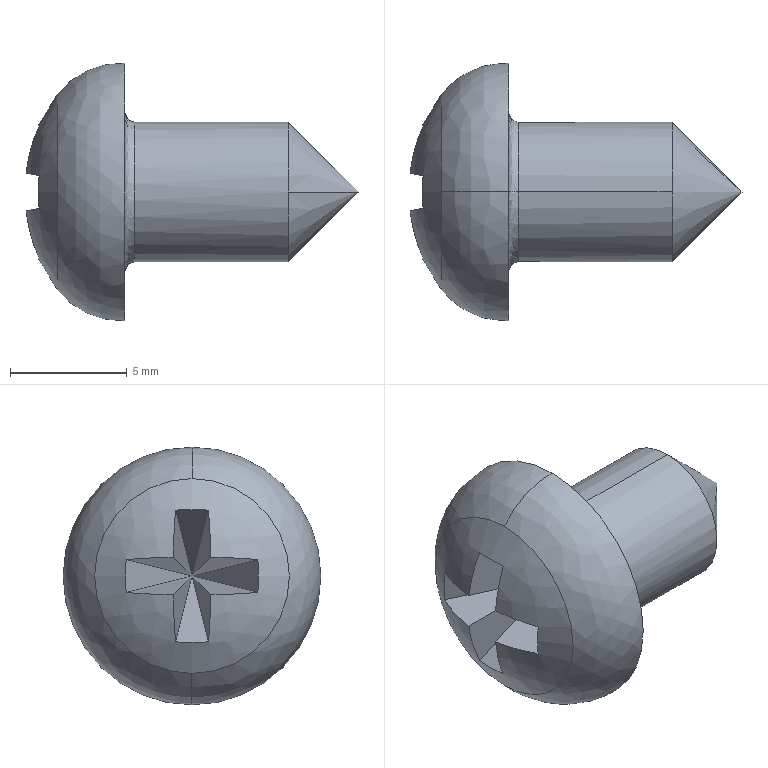Part | SolidWorks | features BaseBody 1, MoveFace 1 | 1 solid | 22 faces | box 14.243 x 11.05 x 11.056 mm | volume 485.827 mm3 | plane 13 | spline 5 | cylinder 2 | cone 2 | commonest cylinder face diameters 6 x2
STEP:
#1=CARTESIAN_POINT('',(4.74,0.,-3.));
#2=VERTEX_POINT('',#1);
#3=CARTESIAN_POINT('',(4.74,0.,3.));
#4=VERTEX_POINT('',#3);
#5=CARTESIAN_POINT('',(4.74,0.,0.));
#6=DIRECTION('',(1.,0.,0.));
#7=DIRECTION('',(0.,0.,1.));
#8=AXIS2_PLACEMENT_3D('',#5,#6,#7);
#9=CIRCLE('',#8,3.);
#10=EDGE_CURVE('',#2,#4,#9,.T.);
#11=ORIENTED_EDGE('',*,*,#10,.F.);
#12=CARTESIAN_POINT('',(4.34,0.,-3.4));
#13=VERTEX_POINT('',#12);
#14=CARTESIAN_POINT('',(4.74,0.,-3.4));
#15=DIRECTION('',(0.,-1.,0.));
#16=DIRECTION('',(0.,0.,-1.));
#17=AXIS2_PLACEMENT_3D('',#14,#15,#16);
#18=CIRCLE('',#17,0.4);
#19=EDGE_CURVE('',#2,#13,#18,.T.);
#20=ORIENTED_EDGE('',*,*,#19,.T.);
#21=CARTESIAN_POINT('',(4.34,0.,3.4));
#22=VERTEX_POINT('',#21);
#23=CARTESIAN_POINT('',(4.34,0.,3.4));
#24=CARTESIAN_POINT('',(4.34,0.2163,3.4));
#25=CARTESIAN_POINT('',(4.34,0.5349,3.37));
#26=CARTESIAN_POINT('',(4.34,0.8966,3.283));
#27=CARTESIAN_POINT('',(4.34,1.075,3.227));
#28=CARTESIAN_POINT('',(4.34,1.163,3.195));
#29=CARTESIAN_POINT('',(4.34,1.201,3.181));
#30=CARTESIAN_POINT('',(4.34,1.226,3.171));
#31=CARTESIAN_POINT('',(4.34,1.238,3.167));
#32=CARTESIAN_POINT('',(4.34,1.688,2.988));
#33=CARTESIAN_POINT('',(4.34,2.072,2.736));
#34=CARTESIAN_POINT('',(4.34,2.57,2.238));
#35=CARTESIAN_POINT('',(4.34,2.789,1.969));
#36=CARTESIAN_POINT('',(4.34,2.993,1.622));
#37=CARTESIAN_POINT('',(4.34,3.081,1.44));
#38=CARTESIAN_POINT('',(4.34,3.122,1.346));
#39=CARTESIAN_POINT('',(4.34,3.139,1.306));
#40=CARTESIAN_POINT('',(4.34,3.15,1.279));
#41=CARTESIAN_POINT('',(4.34,3.156,1.264));
#42=CARTESIAN_POINT('',(4.34,3.32,0.8492));
#43=CARTESIAN_POINT('',(4.34,3.4,0.4327));
#44=CARTESIAN_POINT('',(4.34,3.4,-0.2164));
#45=CARTESIAN_POINT('',(4.34,3.37,-0.5351));
#46=CARTESIAN_POINT('',(4.34,3.283,-0.8967));
#47=CARTESIAN_POINT('',(4.34,3.227,-1.075));
#48=CARTESIAN_POINT('',(4.34,3.195,-1.163));
#49=CARTESIAN_POINT('',(4.34,3.181,-1.201));
#50=CARTESIAN_POINT('',(4.34,3.171,-1.226));
#51=CARTESIAN_POINT('',(4.34,3.167,-1.238));
#52=CARTESIAN_POINT('',(4.34,2.988,-1.688));
#53=CARTESIAN_POINT('',(4.34,2.736,-2.072));
#54=CARTESIAN_POINT('',(4.34,2.238,-2.57));
#55=CARTESIAN_POINT('',(4.34,1.969,-2.789));
#56=CARTESIAN_POINT('',(4.34,1.622,-2.993));
#57=CARTESIAN_POINT('',(4.34,1.44,-3.081));
#58=CARTESIAN_POINT('',(4.34,1.346,-3.122));
#59=CARTESIAN_POINT('',(4.34,1.306,-3.139));
#60=CARTESIAN_POINT('',(4.34,1.279,-3.15));
#61=CARTESIAN_POINT('',(4.34,1.264,-3.156));
#62=CARTESIAN_POINT('',(4.34,0.8493,-3.32));
#63=CARTESIAN_POINT('',(4.34,0.4322,-3.4));
#64=CARTESIAN_POINT('',(4.34,0.,-3.4));
#65=B_SPLINE_CURVE_WITH_KNOTS('',3,(#23,#24,#25,#26,#27,#28,#29,#30,#31,#32,#33,#34,#35,#36,#37,#38,#39,#40,#41,#42,#43,#44,#45,#46,#47,#48,#49,#50,#51,#52,#53,#54,#55,#56,#57,#58,#59,#60,#61,#62,#63,#64),.UNSPECIFIED.,.F.,.F.,(4,1,1,1,1,2,2,2,1,1,1,1,2,2,2,1,1,1,1,2,2,2,1,1,1,1,2,2,4),(0.,0.0625,0.09375,0.1094,0.1172,0.1211,0.125,0.25,0.3125,0.3437,0.3594,0.3672,0.3711,0.375,0.5,0.5625,0.5937,0.6094,0.6172,0.6211,0.625,0.75,0.8125,0.8437,0.8594,0.8672,0.8711,0.875,1.),.UNSPECIFIED.);
#66=EDGE_CURVE('',#22,#13,#65,.T.);
#67=ORIENTED_EDGE('',*,*,#66,.F.);
#68=CARTESIAN_POINT('',(4.74,0.,3.4));
#69=DIRECTION('',(0.,1.,0.));
#70=DIRECTION('',(0.,0.,1.));
#71=AXIS2_PLACEMENT_3D('',#68,#69,#70);
#72=CIRCLE('',#71,0.4);
#73=EDGE_CURVE('',#4,#22,#72,.T.);
#74=ORIENTED_EDGE('',*,*,#73,.F.);
#75=EDGE_LOOP('',(#11,#20,#67,#74));
#76=FACE_OUTER_BOUND('',#75,.T.);
#77=CARTESIAN_POINT('',(4.74,0.,3.));
#78=CARTESIAN_POINT('',(4.74,6.,3.));
#79=CARTESIAN_POINT('',(4.74,6.,-3.));
#80=CARTESIAN_POINT('',(4.74,0.,-3.));
#81=CARTESIAN_POINT('',(4.506,0.,3.));
#82=CARTESIAN_POINT('',(4.506,6.,3.));
#83=CARTESIAN_POINT('',(4.506,6.,-3.));
#84=CARTESIAN_POINT('',(4.506,0.,-3.));
#85=CARTESIAN_POINT('',(4.34,0.,3.166));
#86=CARTESIAN_POINT('',(4.34,6.331,3.166));
#87=CARTESIAN_POINT('',(4.34,6.331,-3.166));
#88=CARTESIAN_POINT('',(4.34,0.,-3.166));
#89=CARTESIAN_POINT('',(4.34,0.,3.4));
#90=CARTESIAN_POINT('',(4.34,6.8,3.4));
#91=CARTESIAN_POINT('',(4.34,6.8,-3.4));
#92=CARTESIAN_POINT('',(4.34,0.,-3.4));
#93=(BOUNDED_SURFACE()B_SPLINE_SURFACE(3,3,((#77,#78,#79,#80),(#81,#82,#83,#84),(#85,#86,#87,#88),(#89,#90,#91,#92)),.UNSPECIFIED.,.F.,.F.,.F.)B_SPLINE_SURFACE_WITH_KNOTS((4,4),(4,4),(0.,1.),(0.,1.),.UNSPECIFIED.)GEOMETRIC_REPRESENTATION_ITEM()RATIONAL_B_SPLINE_SURFACE(((1.,0.3333,0.3333,1.),(0.8047,0.2682,0.2682,0.8047),(0.8047,0.2682,0.2682,0.8047),(1.,0.3333,0.3333,1.)))REPRESENTATION_ITEM('')SURFACE());
#94=ADVANCED_FACE('',(#76),#93,.F.);
#95=CARTESIAN_POINT('',(1.436,0.,4.179));
#96=VERTEX_POINT('',#95);
#97=CARTESIAN_POINT('',(1.436,0.,-4.179));
#98=VERTEX_POINT('',#97);
#99=CARTESIAN_POINT('',(1.436,0.,0.));
#100=DIRECTION('',(1.,0.,0.));
#101=DIRECTION('',(0.,0.,1.));
#102=AXIS2_PLACEMENT_3D('',#99,#100,#101);
#103=CIRCLE('',#102,4.179);
#104=EDGE_CURVE('',#96,#98,#103,.T.);
#105=ORIENTED_EDGE('',*,*,#104,.T.);
#106=CARTESIAN_POINT('',(4.34,0.,-5.525));
#107=VERTEX_POINT('',#106);
#108=CARTESIAN_POINT('',(4.197,0.,-2.028));
#109=DIRECTION('',(0.,-1.,0.));
#110=DIRECTION('',(0.,0.,-1.));
#111=AXIS2_PLACEMENT_3D('',#108,#109,#110);
#112=CIRCLE('',#111,3.5);
#113=EDGE_CURVE('',#98,#107,#112,.T.);
#114=ORIENTED_EDGE('',*,*,#113,.T.);
#115=CARTESIAN_POINT('',(4.34,0.,5.525));
#116=VERTEX_POINT('',#115);
#117=CARTESIAN_POINT('',(4.34,0.,0.));
#118=DIRECTION('',(-1.,0.,0.));
#119=DIRECTION('',(0.,0.,1.));
#120=AXIS2_PLACEMENT_3D('',#117,#118,#119);
#121=CIRCLE('',#120,5.525);
#122=EDGE_CURVE('',#107,#116,#121,.T.);
#123=ORIENTED_EDGE('',*,*,#122,.T.);
#124=CARTESIAN_POINT('',(4.197,0.,2.028));
#125=DIRECTION('',(0.,1.,0.));
#126=DIRECTION('',(0.,0.,1.));
#127=AXIS2_PLACEMENT_3D('',#124,#125,#126);
#128=CIRCLE('',#127,3.5);
#129=EDGE_CURVE('',#96,#116,#128,.T.);
#130=ORIENTED_EDGE('',*,*,#129,.F.);
#131=EDGE_LOOP('',(#105,#114,#123,#130));
#132=FACE_OUTER_BOUND('',#131,.T.);
#133=CARTESIAN_POINT('',(1.436,0.,-4.179));
#134=CARTESIAN_POINT('',(1.436,-8.358,-4.179));
#135=CARTESIAN_POINT('',(1.436,-8.358,4.179));
#136=CARTESIAN_POINT('',(1.436,0.,4.179));
#137=CARTESIAN_POINT('',(2.144,0.,-5.088));
#138=CARTESIAN_POINT('',(2.144,-10.175,-5.088));
#139=CARTESIAN_POINT('',(2.144,-10.175,5.088));
#140=CARTESIAN_POINT('',(2.144,0.,5.088));
#141=CARTESIAN_POINT('',(3.189,0.,-5.572));
#142=CARTESIAN_POINT('',(3.189,-11.144,-5.572));
#143=CARTESIAN_POINT('',(3.189,-11.144,5.572));
#144=CARTESIAN_POINT('',(3.189,0.,5.572));
#145=CARTESIAN_POINT('',(4.34,0.,-5.525));
#146=CARTESIAN_POINT('',(4.34,-11.05,-5.525));
#147=CARTESIAN_POINT('',(4.34,-11.05,5.525));
#148=CARTESIAN_POINT('',(4.34,0.,5.525));
#149=(BOUNDED_SURFACE()B_SPLINE_SURFACE(3,3,((#133,#134,#135,#136),(#137,#138,#139,#140),(#141,#142,#143,#144),(#145,#146,#147,#148)),.UNSPECIFIED.,.F.,.F.,.F.)B_SPLINE_SURFACE_WITH_KNOTS((4,4),(4,4),(0.,1.),(0.,1.),.UNSPECIFIED.)GEOMETRIC_REPRESENTATION_ITEM()RATIONAL_B_SPLINE_SURFACE(((1.,0.3333,0.3333,1.),(0.9262,0.3087,0.3087,0.9262),(0.9262,0.3087,0.3087,0.9262),(1.,0.3333,0.3333,1.)))REPRESENTATION_ITEM('')SURFACE());
#150=ADVANCED_FACE('',(#132),#149,.T.);
#151=CARTESIAN_POINT('',(11.34,3.,0.));
#152=VERTEX_POINT('',#151);
#153=CARTESIAN_POINT('',(11.34,0.,-3.));
#154=VERTEX_POINT('',#153);
#155=CARTESIAN_POINT('',(11.34,0.,0.));
#156=DIRECTION('',(-1.,0.,0.));
#157=DIRECTION('',(0.,0.,1.));
#158=AXIS2_PLACEMENT_3D('',#155,#156,#157);
#159=CIRCLE('',#158,3.);
#160=EDGE_CURVE('',#152,#154,#159,.T.);
#161=ORIENTED_EDGE('',*,*,#160,.T.);
#162=CARTESIAN_POINT('',(-13.629,0.,-3.));
#163=DIRECTION('',(-1.,0.,0.));
#164=VECTOR('',#163,1000.);
#165=LINE('',#162,#164);
#166=EDGE_CURVE('',#154,#2,#165,.T.);
#167=ORIENTED_EDGE('',*,*,#166,.T.);
#168=ORIENTED_EDGE('',*,*,#10,.T.);
#169=CARTESIAN_POINT('',(11.34,0.,3.));
#170=VERTEX_POINT('',#169);
#171=CARTESIAN_POINT('',(-13.629,0.,3.));
#172=DIRECTION('',(-1.,0.,0.));
#173=VECTOR('',#172,1000.);
#174=LINE('',#171,#173);
#175=EDGE_CURVE('',#170,#4,#174,.T.);
#176=ORIENTED_EDGE('',*,*,#175,.F.);
#177=CARTESIAN_POINT('',(11.34,0.,0.));
#178=DIRECTION('',(-1.,0.,0.));
#179=DIRECTION('',(0.,0.,1.));
#180=AXIS2_PLACEMENT_3D('',#177,#178,#179);
#181=CIRCLE('',#180,3.);
#182=EDGE_CURVE('',#170,#152,#181,.T.);
#183=ORIENTED_EDGE('',*,*,#182,.T.);
#184=EDGE_LOOP('',(#161,#167,#168,#176,#183));
#185=FACE_OUTER_BOUND('',#184,.T.);
#186=CARTESIAN_POINT('',(-13.629,0.,0.));
#187=DIRECTION('',(-1.,0.,0.));
#188=DIRECTION('',(0.,0.,1.));
#189=AXIS2_PLACEMENT_3D('',#186,#187,#188);
#190=CYLINDRICAL_SURFACE('',#189,3.);
#191=ADVANCED_FACE('',(#185),#190,.T.);
#192=CARTESIAN_POINT('',(14.34,0.,0.));
#193=VERTEX_POINT('',#192);
#194=CARTESIAN_POINT('',(11.34,-3.,0.));
#195=VERTEX_POINT('',#194);
#196=CARTESIAN_POINT('',(11.34,-3.,0.));
#197=DIRECTION('',(-0.7071,-0.7071,0.));
#198=VECTOR('',#197,1000.);
#199=LINE('',#196,#198);
#200=EDGE_CURVE('',#193,#195,#199,.T.);
#201=ORIENTED_EDGE('',*,*,#200,.F.);
#202=CARTESIAN_POINT('',(11.34,3.,0.));
#203=DIRECTION('',(-0.7071,0.7071,0.));
#204=VECTOR('',#203,1000.);
#205=LINE('',#202,#204);
#206=EDGE_CURVE('',#193,#152,#205,.T.);
#207=ORIENTED_EDGE('',*,*,#206,.T.);
#208=ORIENTED_EDGE('',*,*,#182,.F.);
#209=CARTESIAN_POINT('',(11.34,0.,0.));
#210=DIRECTION('',(-1.,0.,0.));
#211=DIRECTION('',(0.,0.,1.));
#212=AXIS2_PLACEMENT_3D('',#209,#210,#211);
#213=CIRCLE('',#212,3.);
#214=EDGE_CURVE('',#195,#170,#213,.T.);
#215=ORIENTED_EDGE('',*,*,#214,.F.);
#216=EDGE_LOOP('',(#201,#207,#208,#215));
#217=FACE_OUTER_BOUND('',#216,.T.);
#218=CARTESIAN_POINT('',(11.34,0.,0.));
#219=DIRECTION('',(-1.,0.,0.));
#220=DIRECTION('',(0.,-1.,0.));
#221=AXIS2_PLACEMENT_3D('',#218,#219,#220);
#222=CONICAL_SURFACE('',#221,3.,0.7854);
#223=ADVANCED_FACE('',(#217),#222,.T.);
#224=ORIENTED_EDGE('',*,*,#166,.F.);
#225=CARTESIAN_POINT('',(11.34,0.,0.));
#226=DIRECTION('',(-1.,0.,0.));
#227=DIRECTION('',(0.,0.,1.));
#228=AXIS2_PLACEMENT_3D('',#225,#226,#227);
#229=CIRCLE('',#228,3.);
#230=EDGE_CURVE('',#154,#195,#229,.T.);
#231=ORIENTED_EDGE('',*,*,#230,.T.);
#232=ORIENTED_EDGE('',*,*,#214,.T.);
#233=ORIENTED_EDGE('',*,*,#175,.T.);
#234=CARTESIAN_POINT('',(4.74,0.,0.));
#235=DIRECTION('',(1.,0.,0.));
#236=DIRECTION('',(0.,0.,1.));
#237=AXIS2_PLACEMENT_3D('',#234,#235,#236);
#238=CIRCLE('',#237,3.);
#239=EDGE_CURVE('',#4,#2,#238,.T.);
#240=ORIENTED_EDGE('',*,*,#239,.T.);
#241=EDGE_LOOP('',(#224,#231,#232,#233,#240));
#242=FACE_OUTER_BOUND('',#241,.T.);
#243=CARTESIAN_POINT('',(-13.629,0.,0.));
#244=DIRECTION('',(-1.,0.,0.));
#245=DIRECTION('',(0.,0.,1.));
#246=AXIS2_PLACEMENT_3D('',#243,#244,#245);
#247=CYLINDRICAL_SURFACE('',#246,3.);
#248=ADVANCED_FACE('',(#242),#247,.T.);
#249=ORIENTED_EDGE('',*,*,#19,.F.);
#250=ORIENTED_EDGE('',*,*,#239,.F.);
#251=ORIENTED_EDGE('',*,*,#73,.T.);
#252=CARTESIAN_POINT('',(4.34,0.,-3.4));
#253=CARTESIAN_POINT('',(4.34,-0.2163,-3.4));
#254=CARTESIAN_POINT('',(4.34,-0.5349,-3.37));
#255=CARTESIAN_POINT('',(4.34,-0.8966,-3.283));
#256=CARTESIAN_POINT('',(4.34,-1.075,-3.227));
#257=CARTESIAN_POINT('',(4.34,-1.163,-3.195));
#258=CARTESIAN_POINT('',(4.34,-1.201,-3.181));
#259=CARTESIAN_POINT('',(4.34,-1.226,-3.171));
#260=CARTESIAN_POINT('',(4.34,-1.238,-3.167));
#261=CARTESIAN_POINT('',(4.34,-1.688,-2.988));
#262=CARTESIAN_POINT('',(4.34,-2.072,-2.736));
#263=CARTESIAN_POINT('',(4.34,-2.57,-2.238));
#264=CARTESIAN_POINT('',(4.34,-2.789,-1.969));
#265=CARTESIAN_POINT('',(4.34,-2.993,-1.622));
#266=CARTESIAN_POINT('',(4.34,-3.081,-1.44));
#267=CARTESIAN_POINT('',(4.34,-3.122,-1.346));
#268=CARTESIAN_POINT('',(4.34,-3.139,-1.306));
#269=CARTESIAN_POINT('',(4.34,-3.15,-1.279));
#270=CARTESIAN_POINT('',(4.34,-3.156,-1.264));
#271=CARTESIAN_POINT('',(4.34,-3.32,-0.8492));
#272=CARTESIAN_POINT('',(4.34,-3.4,-0.4327));
#273=CARTESIAN_POINT('',(4.34,-3.4,0.2164));
#274=CARTESIAN_POINT('',(4.34,-3.37,0.5351));
#275=CARTESIAN_POINT('',(4.34,-3.283,0.8967));
#276=CARTESIAN_POINT('',(4.34,-3.227,1.075));
#277=CARTESIAN_POINT('',(4.34,-3.195,1.163));
#278=CARTESIAN_POINT('',(4.34,-3.181,1.201));
#279=CARTESIAN_POINT('',(4.34,-3.171,1.226));
#280=CARTESIAN_POINT('',(4.34,-3.167,1.238));
#281=CARTESIAN_POINT('',(4.34,-2.988,1.688));
#282=CARTESIAN_POINT('',(4.34,-2.736,2.072));
#283=CARTESIAN_POINT('',(4.34,-2.238,2.57));
#284=CARTESIAN_POINT('',(4.34,-1.969,2.789));
#285=CARTESIAN_POINT('',(4.34,-1.622,2.993));
#286=CARTESIAN_POINT('',(4.34,-1.44,3.081));
#287=CARTESIAN_POINT('',(4.34,-1.346,3.122));
#288=CARTESIAN_POINT('',(4.34,-1.306,3.139));
#289=CARTESIAN_POINT('',(4.34,-1.279,3.15));
#290=CARTESIAN_POINT('',(4.34,-1.264,3.156));
#291=CARTESIAN_POINT('',(4.34,-0.8493,3.32));
#292=CARTESIAN_POINT('',(4.34,-0.4322,3.4));
#293=CARTESIAN_POINT('',(4.34,0.,3.4));
#294=B_SPLINE_CURVE_WITH_KNOTS('',3,(#252,#253,#254,#255,#256,#257,#258,#259,#260,#261,#262,#263,#264,#265,#266,#267,#268,#269,#270,#271,#272,#273,#274,#275,#276,#277,#278,#279,#280,#281,#282,#283,#284,#285,#286,#287,#288,#289,#290,#291,#292,#293),.UNSPECIFIED.,.F.,.F.,(4,1,1,1,1,2,2,2,1,1,1,1,2,2,2,1,1,1,1,2,2,2,1,1,1,1,2,2,4),(0.,0.0625,0.09375,0.1094,0.1172,0.1211,0.125,0.25,0.3125,0.3437,0.3594,0.3672,0.3711,0.375,0.5,0.5625,0.5937,0.6094,0.6172,0.6211,0.625,0.75,0.8125,0.8437,0.8594,0.8672,0.8711,0.875,1.),.UNSPECIFIED.);
#295=EDGE_CURVE('',#13,#22,#294,.T.);
#296=ORIENTED_EDGE('',*,*,#295,.F.);
#297=EDGE_LOOP('',(#249,#250,#251,#296));
#298=FACE_OUTER_BOUND('',#297,.T.);
#299=CARTESIAN_POINT('',(4.74,0.,-3.));
#300=CARTESIAN_POINT('',(4.74,-6.,-3.));
#301=CARTESIAN_POINT('',(4.74,-6.,3.));
#302=CARTESIAN_POINT('',(4.74,0.,3.));
#303=CARTESIAN_POINT('',(4.506,0.,-3.));
#304=CARTESIAN_POINT('',(4.506,-6.,-3.));
#305=CARTESIAN_POINT('',(4.506,-6.,3.));
#306=CARTESIAN_POINT('',(4.506,0.,3.));
#307=CARTESIAN_POINT('',(4.34,0.,-3.166));
#308=CARTESIAN_POINT('',(4.34,-6.331,-3.166));
#309=CARTESIAN_POINT('',(4.34,-6.331,3.166));
#310=CARTESIAN_POINT('',(4.34,0.,3.166));
#311=CARTESIAN_POINT('',(4.34,0.,-3.4));
#312=CARTESIAN_POINT('',(4.34,-6.8,-3.4));
#313=CARTESIAN_POINT('',(4.34,-6.8,3.4));
#314=CARTESIAN_POINT('',(4.34,0.,3.4));
#315=(BOUNDED_SURFACE()B_SPLINE_SURFACE(3,3,((#299,#300,#301,#302),(#303,#304,#305,#306),(#307,#308,#309,#310),(#311,#312,#313,#314)),.UNSPECIFIED.,.F.,.F.,.F.)B_SPLINE_SURFACE_WITH_KNOTS((4,4),(4,4),(0.,1.),(0.,1.),.UNSPECIFIED.)GEOMETRIC_REPRESENTATION_ITEM()RATIONAL_B_SPLINE_SURFACE(((1.,0.3333,0.3333,1.),(0.8047,0.2682,0.2682,0.8047),(0.8047,0.2682,0.2682,0.8047),(1.,0.3333,0.3333,1.)))REPRESENTATION_ITEM('')SURFACE());
#316=ADVANCED_FACE('',(#298),#315,.F.);
#317=ORIENTED_EDGE('',*,*,#206,.F.);
#318=ORIENTED_EDGE('',*,*,#200,.T.);
#319=ORIENTED_EDGE('',*,*,#230,.F.);
#320=ORIENTED_EDGE('',*,*,#160,.F.);
#321=EDGE_LOOP('',(#317,#318,#319,#320));
#322=FACE_OUTER_BOUND('',#321,.T.);
#323=CARTESIAN_POINT('',(11.34,0.,0.));
#324=DIRECTION('',(-1.,0.,0.));
#325=DIRECTION('',(0.,-1.,0.));
#326=AXIS2_PLACEMENT_3D('',#323,#324,#325);
#327=CONICAL_SURFACE('',#326,3.,0.7854);
#328=ADVANCED_FACE('',(#322),#327,.T.);
#329=CARTESIAN_POINT('',(4.34,0.,0.));
#330=DIRECTION('',(-1.,0.,0.));
#331=DIRECTION('',(0.,0.,1.));
#332=AXIS2_PLACEMENT_3D('',#329,#330,#331);
#333=CIRCLE('',#332,5.525);
#334=EDGE_CURVE('',#116,#107,#333,.T.);
#335=ORIENTED_EDGE('',*,*,#334,.F.);
#336=ORIENTED_EDGE('',*,*,#122,.F.);
#337=EDGE_LOOP('',(#335,#336));
#338=FACE_OUTER_BOUND('',#337,.T.);
#339=ORIENTED_EDGE('',*,*,#295,.T.);
#340=ORIENTED_EDGE('',*,*,#66,.T.);
#341=EDGE_LOOP('',(#339,#340));
#342=FACE_BOUND('',#341,.T.);
#343=CARTESIAN_POINT('',(4.34,0.,-3.));
#344=DIRECTION('',(-1.,0.,0.));
#345=DIRECTION('',(0.,0.,1.));
#346=AXIS2_PLACEMENT_3D('',#343,#344,#345);
#347=PLANE('',#346);
#348=ADVANCED_FACE('',(#338,#342),#347,.F.);
#349=ORIENTED_EDGE('',*,*,#113,.F.);
#350=CARTESIAN_POINT('',(1.436,0.,0.));
#351=DIRECTION('',(1.,0.,0.));
#352=DIRECTION('',(0.,0.,1.));
#353=AXIS2_PLACEMENT_3D('',#350,#351,#352);
#354=CIRCLE('',#353,4.179);
#355=EDGE_CURVE('',#98,#96,#354,.T.);
#356=ORIENTED_EDGE('',*,*,#355,.T.);
#357=ORIENTED_EDGE('',*,*,#129,.T.);
#358=ORIENTED_EDGE('',*,*,#334,.T.);
#359=EDGE_LOOP('',(#349,#356,#357,#358));
#360=FACE_OUTER_BOUND('',#359,.T.);
#361=CARTESIAN_POINT('',(1.436,0.,4.179));
#362=CARTESIAN_POINT('',(1.436,8.358,4.179));
#363=CARTESIAN_POINT('',(1.436,8.358,-4.179));
#364=CARTESIAN_POINT('',(1.436,0.,-4.179));
#365=CARTESIAN_POINT('',(2.144,0.,5.088));
#366=CARTESIAN_POINT('',(2.144,10.175,5.088));
#367=CARTESIAN_POINT('',(2.144,10.175,-5.088));
#368=CARTESIAN_POINT('',(2.144,0.,-5.088));
#369=CARTESIAN_POINT('',(3.189,0.,5.572));
#370=CARTESIAN_POINT('',(3.189,11.144,5.572));
#371=CARTESIAN_POINT('',(3.189,11.144,-5.572));
#372=CARTESIAN_POINT('',(3.189,0.,-5.572));
#373=CARTESIAN_POINT('',(4.34,0.,5.525));
#374=CARTESIAN_POINT('',(4.34,11.05,5.525));
#375=CARTESIAN_POINT('',(4.34,11.05,-5.525));
#376=CARTESIAN_POINT('',(4.34,0.,-5.525));
#377=(BOUNDED_SURFACE()B_SPLINE_SURFACE(3,3,((#361,#362,#363,#364),(#365,#366,#367,#368),(#369,#370,#371,#372),(#373,#374,#375,#376)),.UNSPECIFIED.,.F.,.F.,.F.)B_SPLINE_SURFACE_WITH_KNOTS((4,4),(4,4),(0.,1.),(0.,1.),.UNSPECIFIED.)GEOMETRIC_REPRESENTATION_ITEM()RATIONAL_B_SPLINE_SURFACE(((1.,0.3333,0.3333,1.),(0.9262,0.3087,0.3087,0.9262),(0.9262,0.3087,0.3087,0.9262),(1.,0.3333,0.3333,1.)))REPRESENTATION_ITEM('')SURFACE());
#378=ADVANCED_FACE('',(#360),#377,.T.);
#379=ORIENTED_EDGE('',*,*,#104,.F.);
#380=ORIENTED_EDGE('',*,*,#355,.F.);
#381=EDGE_LOOP('',(#379,#380));
#382=FACE_OUTER_BOUND('',#381,.T.);
#383=CARTESIAN_POINT('',(0.09661,0.8076,0.8076));
#384=VERTEX_POINT('',#383);
#385=CARTESIAN_POINT('',(0.6565,0.707,2.828));
#386=VERTEX_POINT('',#385);
#387=CARTESIAN_POINT('',(0.09661,0.8076,0.8076));
#388=CARTESIAN_POINT('',(0.1795,0.7927,1.511));
#389=CARTESIAN_POINT('',(0.3662,0.7592,2.184));
#390=CARTESIAN_POINT('',(0.6565,0.707,2.828));
#391=B_SPLINE_CURVE_WITH_KNOTS('',3,(#387,#388,#389,#390),.UNSPECIFIED.,.F.,.F.,(4,4),(0.,0.002099),.UNSPECIFIED.);
#392=EDGE_CURVE('',#384,#386,#391,.T.);
#393=ORIENTED_EDGE('',*,*,#392,.T.);
#394=CARTESIAN_POINT('',(0.6565,-0.707,2.828));
#395=VERTEX_POINT('',#394);
#396=CARTESIAN_POINT('',(0.6565,0.707,2.828));
#397=CARTESIAN_POINT('',(0.6159,0.237,2.857));
#398=CARTESIAN_POINT('',(0.6159,-0.237,2.857));
#399=CARTESIAN_POINT('',(0.6565,-0.707,2.828));
#400=B_SPLINE_CURVE_WITH_KNOTS('',3,(#396,#397,#398,#399),.UNSPECIFIED.,.F.,.F.,(4,4),(-0.000708,0.000708),.UNSPECIFIED.);
#401=EDGE_CURVE('',#386,#395,#400,.T.);
#402=ORIENTED_EDGE('',*,*,#401,.T.);
#403=CARTESIAN_POINT('',(0.09661,-0.8076,0.8076));
#404=VERTEX_POINT('',#403);
#405=CARTESIAN_POINT('',(0.6565,-0.707,2.828));
#406=CARTESIAN_POINT('',(0.3662,-0.7592,2.184));
#407=CARTESIAN_POINT('',(0.1795,-0.7927,1.511));
#408=CARTESIAN_POINT('',(0.09661,-0.8076,0.8076));
#409=B_SPLINE_CURVE_WITH_KNOTS('',3,(#405,#406,#407,#408),.UNSPECIFIED.,.F.,.F.,(4,4),(0.,0.002099),.UNSPECIFIED.);
#410=EDGE_CURVE('',#395,#404,#409,.T.);
#411=ORIENTED_EDGE('',*,*,#410,.T.);
#412=CARTESIAN_POINT('',(0.6565,-2.828,0.707));
#413=VERTEX_POINT('',#412);
#414=CARTESIAN_POINT('',(0.09661,-0.8076,0.8076));
#415=CARTESIAN_POINT('',(0.1795,-1.511,0.7927));
#416=CARTESIAN_POINT('',(0.3662,-2.184,0.7592));
#417=CARTESIAN_POINT('',(0.6565,-2.828,0.707));
#418=B_SPLINE_CURVE_WITH_KNOTS('',3,(#414,#415,#416,#417),.UNSPECIFIED.,.F.,.F.,(4,4),(0.,0.002099),.UNSPECIFIED.);
#419=EDGE_CURVE('',#404,#413,#418,.T.);
#420=ORIENTED_EDGE('',*,*,#419,.T.);
#421=CARTESIAN_POINT('',(0.6565,-2.828,-0.707));
#422=VERTEX_POINT('',#421);
#423=CARTESIAN_POINT('',(0.6565,-2.828,0.707));
#424=CARTESIAN_POINT('',(0.6157,-2.857,0.2357));
#425=CARTESIAN_POINT('',(0.6157,-2.857,-0.2357));
#426=CARTESIAN_POINT('',(0.6565,-2.828,-0.707));
#427=B_SPLINE_CURVE_WITH_KNOTS('',3,(#423,#424,#425,#426),.UNSPECIFIED.,.F.,.F.,(4,4),(0.,0.001414),.UNSPECIFIED.);
#428=EDGE_CURVE('',#413,#422,#427,.T.);
#429=ORIENTED_EDGE('',*,*,#428,.T.);
#430=CARTESIAN_POINT('',(0.09661,-0.8076,-0.8076));
#431=VERTEX_POINT('',#430);
#432=CARTESIAN_POINT('',(0.6565,-2.828,-0.707));
#433=CARTESIAN_POINT('',(0.3662,-2.184,-0.7592));
#434=CARTESIAN_POINT('',(0.1795,-1.511,-0.7927));
#435=CARTESIAN_POINT('',(0.09661,-0.8076,-0.8076));
#436=B_SPLINE_CURVE_WITH_KNOTS('',3,(#432,#433,#434,#435),.UNSPECIFIED.,.F.,.F.,(4,4),(0.,0.002099),.UNSPECIFIED.);
#437=EDGE_CURVE('',#422,#431,#436,.T.);
#438=ORIENTED_EDGE('',*,*,#437,.T.);
#439=CARTESIAN_POINT('',(0.6565,-0.707,-2.828));
#440=VERTEX_POINT('',#439);
#441=CARTESIAN_POINT('',(0.09661,-0.8076,-0.8076));
#442=CARTESIAN_POINT('',(0.1795,-0.7927,-1.511));
#443=CARTESIAN_POINT('',(0.3662,-0.7592,-2.184));
#444=CARTESIAN_POINT('',(0.6565,-0.707,-2.828));
#445=B_SPLINE_CURVE_WITH_KNOTS('',3,(#441,#442,#443,#444),.UNSPECIFIED.,.F.,.F.,(4,4),(0.,0.002099),.UNSPECIFIED.);
#446=EDGE_CURVE('',#431,#440,#445,.T.);
#447=ORIENTED_EDGE('',*,*,#446,.T.);
#448=CARTESIAN_POINT('',(0.6565,0.707,-2.828));
#449=VERTEX_POINT('',#448);
#450=CARTESIAN_POINT('',(0.6565,-0.707,-2.828));
#451=CARTESIAN_POINT('',(0.6159,-0.237,-2.857));
#452=CARTESIAN_POINT('',(0.6159,0.237,-2.857));
#453=CARTESIAN_POINT('',(0.6565,0.707,-2.828));
#454=B_SPLINE_CURVE_WITH_KNOTS('',3,(#450,#451,#452,#453),.UNSPECIFIED.,.F.,.F.,(4,4),(-0.000708,0.000708),.UNSPECIFIED.);
#455=EDGE_CURVE('',#440,#449,#454,.T.);
#456=ORIENTED_EDGE('',*,*,#455,.T.);
#457=CARTESIAN_POINT('',(0.09661,0.8076,-0.8076));
#458=VERTEX_POINT('',#457);
#459=CARTESIAN_POINT('',(0.6565,0.707,-2.828));
#460=CARTESIAN_POINT('',(0.3662,0.7592,-2.184));
#461=CARTESIAN_POINT('',(0.1795,0.7927,-1.511));
#462=CARTESIAN_POINT('',(0.09661,0.8076,-0.8076));
#463=B_SPLINE_CURVE_WITH_KNOTS('',3,(#459,#460,#461,#462),.UNSPECIFIED.,.F.,.F.,(4,4),(0.,0.002099),.UNSPECIFIED.);
#464=EDGE_CURVE('',#449,#458,#463,.T.);
#465=ORIENTED_EDGE('',*,*,#464,.T.);
#466=CARTESIAN_POINT('',(0.6565,2.828,-0.707));
#467=VERTEX_POINT('',#466);
#468=CARTESIAN_POINT('',(0.09661,0.8076,-0.8076));
#469=CARTESIAN_POINT('',(0.1795,1.511,-0.7927));
#470=CARTESIAN_POINT('',(0.3662,2.184,-0.7592));
#471=CARTESIAN_POINT('',(0.6565,2.828,-0.707));
#472=B_SPLINE_CURVE_WITH_KNOTS('',3,(#468,#469,#470,#471),.UNSPECIFIED.,.F.,.F.,(4,4),(0.,0.002099),.UNSPECIFIED.);
#473=EDGE_CURVE('',#458,#467,#472,.T.);
#474=ORIENTED_EDGE('',*,*,#473,.T.);
#475=CARTESIAN_POINT('',(0.6565,2.828,0.707));
#476=VERTEX_POINT('',#475);
#477=CARTESIAN_POINT('',(0.6565,2.828,-0.707));
#478=CARTESIAN_POINT('',(0.6157,2.857,-0.2357));
#479=CARTESIAN_POINT('',(0.6157,2.857,0.2357));
#480=CARTESIAN_POINT('',(0.6565,2.828,0.707));
#481=B_SPLINE_CURVE_WITH_KNOTS('',3,(#477,#478,#479,#480),.UNSPECIFIED.,.F.,.F.,(4,4),(0.,0.001414),.UNSPECIFIED.);
#482=EDGE_CURVE('',#467,#476,#481,.T.);
#483=ORIENTED_EDGE('',*,*,#482,.T.);
#484=CARTESIAN_POINT('',(0.6565,2.828,0.707));
#485=CARTESIAN_POINT('',(0.3662,2.184,0.7592));
#486=CARTESIAN_POINT('',(0.1795,1.511,0.7927));
#487=CARTESIAN_POINT('',(0.09661,0.8076,0.8076));
#488=B_SPLINE_CURVE_WITH_KNOTS('',3,(#484,#485,#486,#487),.UNSPECIFIED.,.F.,.F.,(4,4),(0.,0.002099),.UNSPECIFIED.);
#489=EDGE_CURVE('',#476,#384,#488,.T.);
#490=ORIENTED_EDGE('',*,*,#489,.T.);
#491=EDGE_LOOP('',(#393,#402,#411,#420,#429,#438,#447,#456,#465,#474,#483,#490));
#492=FACE_BOUND('',#491,.T.);
#493=CARTESIAN_POINT('',(2.642,-3.304,-4.246));
#494=CARTESIAN_POINT('',(1.037,-1.284,-4.246));
#495=CARTESIAN_POINT('',(1.039,1.296,-4.246));
#496=CARTESIAN_POINT('',(2.649,3.313,-4.246));
#497=CARTESIAN_POINT('',(1.028,-4.587,-1.668));
#498=CARTESIAN_POINT('',(-1.2,-1.782,-1.668));
#499=CARTESIAN_POINT('',(-1.197,1.799,-1.668));
#500=CARTESIAN_POINT('',(1.037,4.599,-1.668));
#501=CARTESIAN_POINT('',(1.022,-4.591,1.633));
#502=CARTESIAN_POINT('',(-1.209,-1.784,1.633));
#503=CARTESIAN_POINT('',(-1.205,1.801,1.633));
#504=CARTESIAN_POINT('',(1.031,4.604,1.633));
#505=CARTESIAN_POINT('',(2.626,-3.316,4.221));
#506=CARTESIAN_POINT('',(1.015,-1.289,4.221));
#507=CARTESIAN_POINT('',(1.018,1.301,4.221));
#508=CARTESIAN_POINT('',(2.633,3.325,4.221));
#509=(BOUNDED_SURFACE()B_SPLINE_SURFACE(3,3,((#493,#494,#495,#496),(#497,#498,#499,#500),(#501,#502,#503,#504),(#505,#506,#507,#508)),.UNSPECIFIED.,.F.,.F.,.T.)B_SPLINE_SURFACE_WITH_KNOTS((4,4),(4,4),(0.,1.),(0.,1.),.UNSPECIFIED.)GEOMETRIC_REPRESENTATION_ITEM()RATIONAL_B_SPLINE_SURFACE(((1.,0.8549,0.8549,1.),(0.855,0.7309,0.7309,0.855),(0.855,0.7309,0.7309,0.855),(1.,0.8549,0.8549,1.)))REPRESENTATION_ITEM('')SURFACE());
#510=ADVANCED_FACE('',(#382,#492),#509,.T.);
#511=CARTESIAN_POINT('',(4.59,0.,0.));
#512=VERTEX_POINT('',#511);
#513=CARTESIAN_POINT('',(0.6565,0.707,2.828));
#514=DIRECTION('',(0.8034,-0.1444,-0.5776));
#515=VECTOR('',#514,1000.);
#516=LINE('',#513,#515);
#517=EDGE_CURVE('',#386,#512,#516,.T.);
#518=ORIENTED_EDGE('',*,*,#517,.F.);
#519=ORIENTED_EDGE('',*,*,#392,.F.);
#520=CARTESIAN_POINT('',(4.59,0.,0.));
#521=DIRECTION('',(-0.9692,0.1742,0.1742));
#522=VECTOR('',#521,1000.);
#523=LINE('',#520,#522);
#524=EDGE_CURVE('',#512,#384,#523,.T.);
#525=ORIENTED_EDGE('',*,*,#524,.F.);
#526=EDGE_LOOP('',(#518,#519,#525));
#527=FACE_OUTER_BOUND('',#526,.T.);
#528=CARTESIAN_POINT('',(0.,0.825,0.825));
#529=DIRECTION('',(0.1769,0.9842,0.));
#530=DIRECTION('',(-0.9842,0.1769,0.));
#531=AXIS2_PLACEMENT_3D('',#528,#529,#530);
#532=PLANE('',#531);
#533=ADVANCED_FACE('',(#527),#532,.F.);
#534=ORIENTED_EDGE('',*,*,#524,.T.);
#535=ORIENTED_EDGE('',*,*,#489,.F.);
#536=CARTESIAN_POINT('',(4.59,0.,0.));
#537=DIRECTION('',(-0.8034,0.5776,0.1444));
#538=VECTOR('',#537,1000.);
#539=LINE('',#536,#538);
#540=EDGE_CURVE('',#512,#476,#539,.T.);
#541=ORIENTED_EDGE('',*,*,#540,.F.);
#542=EDGE_LOOP('',(#534,#535,#541));
#543=FACE_OUTER_BOUND('',#542,.T.);
#544=CARTESIAN_POINT('',(0.,3.3,0.825));
#545=DIRECTION('',(0.1769,0.,0.9842));
#546=DIRECTION('',(0.9842,0.,-0.1769));
#547=AXIS2_PLACEMENT_3D('',#544,#545,#546);
#548=PLANE('',#547);
#549=ADVANCED_FACE('',(#543),#548,.F.);
#550=CARTESIAN_POINT('',(0.6565,2.828,-0.707));
#551=DIRECTION('',(0.8034,-0.5776,0.1444));
#552=VECTOR('',#551,1000.);
#553=LINE('',#550,#552);
#554=EDGE_CURVE('',#467,#512,#553,.T.);
#555=ORIENTED_EDGE('',*,*,#554,.F.);
#556=ORIENTED_EDGE('',*,*,#473,.F.);
#557=CARTESIAN_POINT('',(4.59,0.,0.));
#558=DIRECTION('',(-0.9692,0.1742,-0.1742));
#559=VECTOR('',#558,1000.);
#560=LINE('',#557,#559);
#561=EDGE_CURVE('',#512,#458,#560,.T.);
#562=ORIENTED_EDGE('',*,*,#561,.F.);
#563=EDGE_LOOP('',(#555,#556,#562));
#564=FACE_OUTER_BOUND('',#563,.T.);
#565=CARTESIAN_POINT('',(0.,0.825,-0.825));
#566=DIRECTION('',(0.1769,0.,-0.9842));
#567=DIRECTION('',(-0.9842,0.,-0.1769));
#568=AXIS2_PLACEMENT_3D('',#565,#566,#567);
#569=PLANE('',#568);
#570=ADVANCED_FACE('',(#564),#569,.F.);
#571=ORIENTED_EDGE('',*,*,#561,.T.);
#572=ORIENTED_EDGE('',*,*,#464,.F.);
#573=CARTESIAN_POINT('',(4.59,0.,0.));
#574=DIRECTION('',(-0.8034,0.1444,-0.5776));
#575=VECTOR('',#574,1000.);
#576=LINE('',#573,#575);
#577=EDGE_CURVE('',#512,#449,#576,.T.);
#578=ORIENTED_EDGE('',*,*,#577,.F.);
#579=EDGE_LOOP('',(#571,#572,#578));
#580=FACE_OUTER_BOUND('',#579,.T.);
#581=CARTESIAN_POINT('',(0.,0.825,-3.3));
#582=DIRECTION('',(0.1769,0.9842,0.));
#583=DIRECTION('',(-0.9842,0.1769,0.));
#584=AXIS2_PLACEMENT_3D('',#581,#582,#583);
#585=PLANE('',#584);
#586=ADVANCED_FACE('',(#580),#585,.F.);
#587=CARTESIAN_POINT('',(0.6565,-0.707,-2.828));
#588=DIRECTION('',(0.8034,0.1444,0.5776));
#589=VECTOR('',#588,1000.);
#590=LINE('',#587,#589);
#591=EDGE_CURVE('',#440,#512,#590,.T.);
#592=ORIENTED_EDGE('',*,*,#591,.F.);
#593=ORIENTED_EDGE('',*,*,#446,.F.);
#594=CARTESIAN_POINT('',(4.59,0.,0.));
#595=DIRECTION('',(-0.9692,-0.1742,-0.1742));
#596=VECTOR('',#595,1000.);
#597=LINE('',#594,#596);
#598=EDGE_CURVE('',#512,#431,#597,.T.);
#599=ORIENTED_EDGE('',*,*,#598,.F.);
#600=EDGE_LOOP('',(#592,#593,#599));
#601=FACE_OUTER_BOUND('',#600,.T.);
#602=CARTESIAN_POINT('',(0.,-0.825,-0.825));
#603=DIRECTION('',(0.1769,-0.9842,0.));
#604=DIRECTION('',(0.9842,0.1769,0.));
#605=AXIS2_PLACEMENT_3D('',#602,#603,#604);
#606=PLANE('',#605);
#607=ADVANCED_FACE('',(#601),#606,.F.);
#608=ORIENTED_EDGE('',*,*,#598,.T.);
#609=ORIENTED_EDGE('',*,*,#437,.F.);
#610=CARTESIAN_POINT('',(4.59,0.,0.));
#611=DIRECTION('',(-0.8034,-0.5776,-0.1444));
#612=VECTOR('',#611,1000.);
#613=LINE('',#610,#612);
#614=EDGE_CURVE('',#512,#422,#613,.T.);
#615=ORIENTED_EDGE('',*,*,#614,.F.);
#616=EDGE_LOOP('',(#608,#609,#615));
#617=FACE_OUTER_BOUND('',#616,.T.);
#618=CARTESIAN_POINT('',(0.,-3.3,-0.825));
#619=DIRECTION('',(0.1769,0.,-0.9842));
#620=DIRECTION('',(-0.9842,0.,-0.1769));
#621=AXIS2_PLACEMENT_3D('',#618,#619,#620);
#622=PLANE('',#621);
#623=ADVANCED_FACE('',(#617),#622,.F.);
#624=CARTESIAN_POINT('',(0.6565,-2.828,0.707));
#625=DIRECTION('',(0.8034,0.5776,-0.1444));
#626=VECTOR('',#625,1000.);
#627=LINE('',#624,#626);
#628=EDGE_CURVE('',#413,#512,#627,.T.);
#629=ORIENTED_EDGE('',*,*,#628,.F.);
#630=ORIENTED_EDGE('',*,*,#419,.F.);
#631=CARTESIAN_POINT('',(4.59,0.,0.));
#632=DIRECTION('',(-0.9692,-0.1742,0.1742));
#633=VECTOR('',#632,1000.);
#634=LINE('',#631,#633);
#635=EDGE_CURVE('',#512,#404,#634,.T.);
#636=ORIENTED_EDGE('',*,*,#635,.F.);
#637=EDGE_LOOP('',(#629,#630,#636));
#638=FACE_OUTER_BOUND('',#637,.T.);
#639=CARTESIAN_POINT('',(0.,-0.825,0.825));
#640=DIRECTION('',(0.1769,0.,0.9842));
#641=DIRECTION('',(0.9842,0.,-0.1769));
#642=AXIS2_PLACEMENT_3D('',#639,#640,#641);
#643=PLANE('',#642);
#644=ADVANCED_FACE('',(#638),#643,.F.);
#645=ORIENTED_EDGE('',*,*,#635,.T.);
#646=ORIENTED_EDGE('',*,*,#410,.F.);
#647=CARTESIAN_POINT('',(4.59,0.,0.));
#648=DIRECTION('',(-0.8034,-0.1444,0.5776));
#649=VECTOR('',#648,1000.);
#650=LINE('',#647,#649);
#651=EDGE_CURVE('',#512,#395,#650,.T.);
#652=ORIENTED_EDGE('',*,*,#651,.F.);
#653=EDGE_LOOP('',(#645,#646,#652));
#654=FACE_OUTER_BOUND('',#653,.T.);
#655=CARTESIAN_POINT('',(0.,-0.825,3.3));
#656=DIRECTION('',(0.1769,-0.9842,0.));
#657=DIRECTION('',(0.9842,0.1769,0.));
#658=AXIS2_PLACEMENT_3D('',#655,#656,#657);
#659=PLANE('',#658);
#660=ADVANCED_FACE('',(#654),#659,.F.);
#661=ORIENTED_EDGE('',*,*,#651,.T.);
#662=ORIENTED_EDGE('',*,*,#401,.F.);
#663=ORIENTED_EDGE('',*,*,#517,.T.);
#664=EDGE_LOOP('',(#661,#662,#663));
#665=FACE_OUTER_BOUND('',#664,.T.);
#666=CARTESIAN_POINT('',(0.,0.825,3.3));
#667=DIRECTION('',(0.5837,0.,0.8119));
#668=DIRECTION('',(0.8119,0.,-0.5837));
#669=AXIS2_PLACEMENT_3D('',#666,#667,#668);
#670=PLANE('',#669);
#671=ADVANCED_FACE('',(#665),#670,.F.);
#672=ORIENTED_EDGE('',*,*,#540,.T.);
#673=ORIENTED_EDGE('',*,*,#482,.F.);
#674=ORIENTED_EDGE('',*,*,#554,.T.);
#675=EDGE_LOOP('',(#672,#673,#674));
#676=FACE_OUTER_BOUND('',#675,.T.);
#677=CARTESIAN_POINT('',(0.,3.3,-0.825));
#678=DIRECTION('',(0.5837,0.8119,0.));
#679=DIRECTION('',(-0.8119,0.5837,0.));
#680=AXIS2_PLACEMENT_3D('',#677,#678,#679);
#681=PLANE('',#680);
#682=ADVANCED_FACE('',(#676),#681,.F.);
#683=ORIENTED_EDGE('',*,*,#577,.T.);
#684=ORIENTED_EDGE('',*,*,#455,.F.);
#685=ORIENTED_EDGE('',*,*,#591,.T.);
#686=EDGE_LOOP('',(#683,#684,#685));
#687=FACE_OUTER_BOUND('',#686,.T.);
#688=CARTESIAN_POINT('',(0.,-0.825,-3.3));
#689=DIRECTION('',(0.5837,0.,-0.8119));
#690=DIRECTION('',(-0.8119,0.,-0.5837));
#691=AXIS2_PLACEMENT_3D('',#688,#689,#690);
#692=PLANE('',#691);
#693=ADVANCED_FACE('',(#687),#692,.F.);
#694=ORIENTED_EDGE('',*,*,#614,.T.);
#695=ORIENTED_EDGE('',*,*,#428,.F.);
#696=ORIENTED_EDGE('',*,*,#628,.T.);
#697=EDGE_LOOP('',(#694,#695,#696));
#698=FACE_OUTER_BOUND('',#697,.T.);
#699=CARTESIAN_POINT('',(0.,-3.3,0.825));
#700=DIRECTION('',(0.5837,-0.8119,0.));
#701=DIRECTION('',(0.8119,0.5837,0.));
#702=AXIS2_PLACEMENT_3D('',#699,#700,#701);
#703=PLANE('',#702);
#704=ADVANCED_FACE('',(#698),#703,.F.);
#705=CLOSED_SHELL('',(#94,#150,#191,#223,#248,#316,#328,#348,#378,#510,#533,#549,#570,#586,#607,#623,#644,#660,#671,#682,#693,#704));
#706=MANIFOLD_SOLID_BREP('',#705);
#707=CARTESIAN_POINT('',(0.,0.,0.));
#708=DIRECTION('',(0.,0.,1.));
#709=DIRECTION('',(1.,0.,0.));
#710=AXIS2_PLACEMENT_3D('',#707,#708,#709);
#711=(LENGTH_UNIT()NAMED_UNIT(*)SI_UNIT(.MILLI.,.METRE.));
#712=UNCERTAINTY_MEASURE_WITH_UNIT(LENGTH_MEASURE(0.00001),#711,'','');
#713=(NAMED_UNIT(*)PLANE_ANGLE_UNIT()SI_UNIT($,.RADIAN.));
#714=(NAMED_UNIT(*)SI_UNIT($,.STERADIAN.)SOLID_ANGLE_UNIT());
#715=(GEOMETRIC_REPRESENTATION_CONTEXT(3)GLOBAL_UNCERTAINTY_ASSIGNED_CONTEXT((#712))GLOBAL_UNIT_ASSIGNED_CONTEXT((#711,#713,#714))REPRESENTATION_CONTEXT('',''));
#716=ADVANCED_BREP_SHAPE_REPRESENTATION('',(#706,#710),#715);